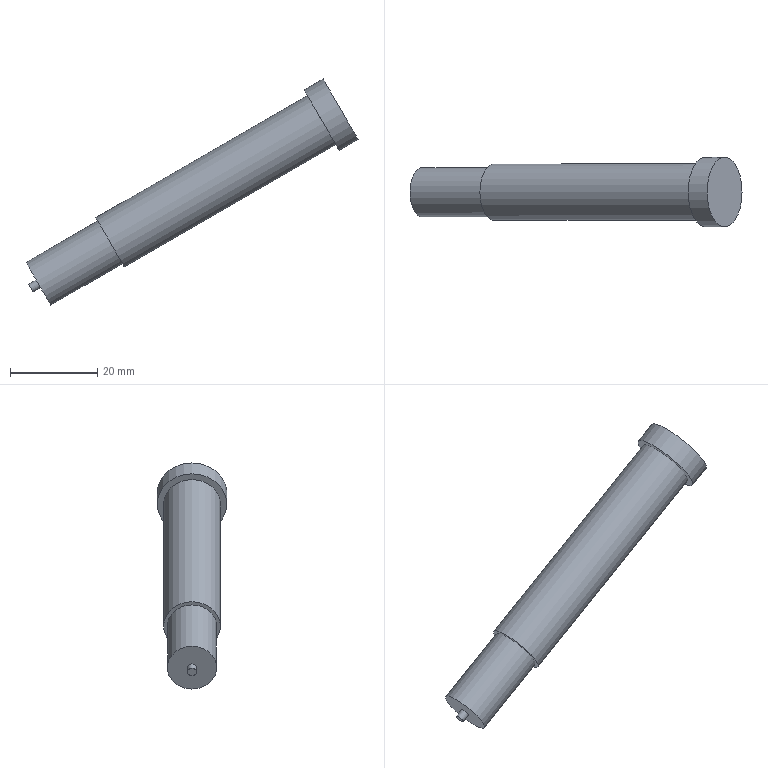Part | NX | features solid 2 | 1 solid | 9 faces | box 76.107 x 16 x 51.821 mm | volume 10350 mm3 | plane 5 | cylinder 4 | commonest cylinder face diameters 2 x1 11.3 x1 13 x1 16 x1
STEP:
#1=CARTESIAN_POINT('',(680.127,-697.825,26.962));
#2=VERTEX_POINT('',#1);
#3=CARTESIAN_POINT('',(683.377,-697.825,21.333));
#4=DIRECTION('',(-0.866,0.00000137,-0.5));
#5=DIRECTION('',(-0.5,0.000000963,0.866));
#6=AXIS2_PLACEMENT_3D('',#3,#4,#5);
#7=CIRCLE('',#6,6.5);
#8=EDGE_CURVE('',#2,#2,#7,.T.);
#9=ORIENTED_EDGE('',*,*,#8,.F.);
#10=EDGE_LOOP('',(#9));
#11=FACE_BOUND('',#10,.T.);
#12=CARTESIAN_POINT('',(728.625,-697.825,54.962));
#13=VERTEX_POINT('',#12);
#14=CARTESIAN_POINT('',(731.875,-697.825,49.333));
#15=DIRECTION('',(-0.866,0.00000137,-0.5));
#16=DIRECTION('',(-0.5,0.000000963,0.866));
#17=AXIS2_PLACEMENT_3D('',#14,#15,#16);
#18=CIRCLE('',#17,6.5);
#19=EDGE_CURVE('',#13,#13,#18,.T.);
#20=ORIENTED_EDGE('',*,*,#19,.T.);
#21=EDGE_LOOP('',(#20));
#22=FACE_BOUND('',#21,.T.);
#23=CARTESIAN_POINT('',(736.205,-697.825,51.833));
#24=DIRECTION('',(-0.866,0.00000137,-0.5));
#25=DIRECTION('',(0.5,-0.000000963,-0.866));
#26=AXIS2_PLACEMENT_3D('',#23,#24,#25);
#27=CYLINDRICAL_SURFACE('',#26,6.5);
#28=ADVANCED_FACE('',(#11,#22),#27,.T.);
#29=CARTESIAN_POINT('',(680.552,-697.825,26.226));
#30=VERTEX_POINT('',#29);
#31=CARTESIAN_POINT('',(683.377,-697.825,21.333));
#32=DIRECTION('',(-0.866,0.00000137,-0.5));
#33=DIRECTION('',(-0.5,0.000000963,0.866));
#34=AXIS2_PLACEMENT_3D('',#31,#32,#33);
#35=CIRCLE('',#34,5.65);
#36=EDGE_CURVE('',#30,#30,#35,.T.);
#37=ORIENTED_EDGE('',*,*,#36,.F.);
#38=EDGE_LOOP('',(#37));
#39=FACE_BOUND('',#38,.T.);
#40=ORIENTED_EDGE('',*,*,#8,.T.);
#41=EDGE_LOOP('',(#40));
#42=FACE_BOUND('',#41,.T.);
#43=CARTESIAN_POINT('',(683.377,-697.825,21.333));
#44=DIRECTION('',(0.866,-0.00000137,0.5));
#45=DIRECTION('',(-0.5,0.000000963,0.866));
#46=AXIS2_PLACEMENT_3D('',#43,#44,#45);
#47=PLANE('',#46);
#48=ADVANCED_FACE('',(#39,#42),#47,.F.);
#49=CARTESIAN_POINT('',(727.875,-697.825,56.261));
#50=VERTEX_POINT('',#49);
#51=CARTESIAN_POINT('',(731.875,-697.825,49.333));
#52=DIRECTION('',(-0.866,0.00000137,-0.5));
#53=DIRECTION('',(-0.5,0.000000963,0.866));
#54=AXIS2_PLACEMENT_3D('',#51,#52,#53);
#55=CIRCLE('',#54,8.);
#56=EDGE_CURVE('',#50,#50,#55,.T.);
#57=ORIENTED_EDGE('',*,*,#56,.T.);
#58=EDGE_LOOP('',(#57));
#59=FACE_BOUND('',#58,.T.);
#60=ORIENTED_EDGE('',*,*,#19,.F.);
#61=EDGE_LOOP('',(#60));
#62=FACE_BOUND('',#61,.T.);
#63=CARTESIAN_POINT('',(731.875,-697.825,49.333));
#64=DIRECTION('',(0.866,-0.00000137,0.5));
#65=DIRECTION('',(-0.5,0.000000963,0.866));
#66=AXIS2_PLACEMENT_3D('',#63,#64,#65);
#67=PLANE('',#66);
#68=ADVANCED_FACE('',(#59,#62),#67,.F.);
#69=ORIENTED_EDGE('',*,*,#56,.F.);
#70=EDGE_LOOP('',(#69));
#71=FACE_BOUND('',#70,.T.);
#72=CARTESIAN_POINT('',(732.205,-697.825,58.761));
#73=VERTEX_POINT('',#72);
#74=CARTESIAN_POINT('',(736.205,-697.825,51.833));
#75=DIRECTION('',(-0.866,0.00000137,-0.5));
#76=DIRECTION('',(-0.5,0.000000963,0.866));
#77=AXIS2_PLACEMENT_3D('',#74,#75,#76);
#78=CIRCLE('',#77,8.);
#79=EDGE_CURVE('',#73,#73,#78,.T.);
#80=ORIENTED_EDGE('',*,*,#79,.T.);
#81=EDGE_LOOP('',(#80));
#82=FACE_BOUND('',#81,.T.);
#83=CARTESIAN_POINT('',(731.875,-697.825,49.333));
#84=DIRECTION('',(0.866,-0.00000137,0.5));
#85=DIRECTION('',(-0.5,0.000000963,0.866));
#86=AXIS2_PLACEMENT_3D('',#83,#84,#85);
#87=CYLINDRICAL_SURFACE('',#86,8.);
#88=ADVANCED_FACE('',(#71,#82),#87,.T.);
#89=ORIENTED_EDGE('',*,*,#79,.F.);
#90=EDGE_LOOP('',(#89));
#91=FACE_BOUND('',#90,.T.);
#92=CARTESIAN_POINT('',(736.205,-697.825,51.833));
#93=DIRECTION('',(0.866,-0.00000137,0.5));
#94=DIRECTION('',(-0.5,0.000000963,0.866));
#95=AXIS2_PLACEMENT_3D('',#92,#93,#94);
#96=PLANE('',#95);
#97=ADVANCED_FACE('',(#91),#96,.T.);
#98=CARTESIAN_POINT('',(664.098,-697.825,16.726));
#99=VERTEX_POINT('',#98);
#100=CARTESIAN_POINT('',(666.923,-697.825,11.833));
#101=DIRECTION('',(-0.866,0.00000137,-0.5));
#102=DIRECTION('',(-0.5,0.000000963,0.866));
#103=AXIS2_PLACEMENT_3D('',#100,#101,#102);
#104=CIRCLE('',#103,5.65);
#105=EDGE_CURVE('',#99,#99,#104,.T.);
#106=ORIENTED_EDGE('',*,*,#105,.F.);
#107=EDGE_LOOP('',(#106));
#108=FACE_BOUND('',#107,.T.);
#109=ORIENTED_EDGE('',*,*,#36,.T.);
#110=EDGE_LOOP('',(#109));
#111=FACE_BOUND('',#110,.T.);
#112=CARTESIAN_POINT('',(666.923,-697.825,11.833));
#113=DIRECTION('',(0.866,-0.00000137,0.5));
#114=DIRECTION('',(-0.5,0.000000963,0.866));
#115=AXIS2_PLACEMENT_3D('',#112,#113,#114);
#116=CYLINDRICAL_SURFACE('',#115,5.65);
#117=ADVANCED_FACE('',(#108,#111),#116,.T.);
#118=CARTESIAN_POINT('',(666.423,-697.825,12.699));
#119=VERTEX_POINT('',#118);
#120=CARTESIAN_POINT('',(666.923,-697.825,11.833));
#121=DIRECTION('',(-0.866,0.00000137,-0.5));
#122=DIRECTION('',(-0.5,0.000000963,0.866));
#123=AXIS2_PLACEMENT_3D('',#120,#121,#122);
#124=CIRCLE('',#123,1.);
#125=EDGE_CURVE('',#119,#119,#124,.T.);
#126=ORIENTED_EDGE('',*,*,#125,.F.);
#127=EDGE_LOOP('',(#126));
#128=FACE_BOUND('',#127,.T.);
#129=ORIENTED_EDGE('',*,*,#105,.T.);
#130=EDGE_LOOP('',(#129));
#131=FACE_BOUND('',#130,.T.);
#132=CARTESIAN_POINT('',(666.923,-697.825,11.833));
#133=DIRECTION('',(0.866,-0.00000137,0.5));
#134=DIRECTION('',(-0.5,0.000000963,0.866));
#135=AXIS2_PLACEMENT_3D('',#132,#133,#134);
#136=PLANE('',#135);
#137=ADVANCED_FACE('',(#128,#131),#136,.F.);
#138=CARTESIAN_POINT('',(664.691,-697.825,11.699));
#139=VERTEX_POINT('',#138);
#140=CARTESIAN_POINT('',(665.191,-697.825,10.833));
#141=DIRECTION('',(-0.866,0.00000137,-0.5));
#142=DIRECTION('',(-0.5,0.000000963,0.866));
#143=AXIS2_PLACEMENT_3D('',#140,#141,#142);
#144=CIRCLE('',#143,1.);
#145=EDGE_CURVE('',#139,#139,#144,.T.);
#146=ORIENTED_EDGE('',*,*,#145,.F.);
#147=EDGE_LOOP('',(#146));
#148=FACE_BOUND('',#147,.T.);
#149=ORIENTED_EDGE('',*,*,#125,.T.);
#150=EDGE_LOOP('',(#149));
#151=FACE_BOUND('',#150,.T.);
#152=CARTESIAN_POINT('',(665.191,-697.825,10.833));
#153=DIRECTION('',(0.866,-0.00000137,0.5));
#154=DIRECTION('',(-0.5,0.000000963,0.866));
#155=AXIS2_PLACEMENT_3D('',#152,#153,#154);
#156=CYLINDRICAL_SURFACE('',#155,1.);
#157=ADVANCED_FACE('',(#148,#151),#156,.T.);
#158=ORIENTED_EDGE('',*,*,#145,.T.);
#159=EDGE_LOOP('',(#158));
#160=FACE_BOUND('',#159,.T.);
#161=CARTESIAN_POINT('',(665.191,-697.825,10.833));
#162=DIRECTION('',(0.866,-0.00000137,0.5));
#163=DIRECTION('',(-0.5,0.000000963,0.866));
#164=AXIS2_PLACEMENT_3D('',#161,#162,#163);
#165=PLANE('',#164);
#166=ADVANCED_FACE('',(#160),#165,.F.);
#167=CLOSED_SHELL('',(#28,#48,#68,#88,#97,#117,#137,#157,#166));
#168=MANIFOLD_SOLID_BREP('',#167);
#169=(LENGTH_UNIT()NAMED_UNIT(*)SI_UNIT(.MILLI.,.METRE.));
#170=UNCERTAINTY_MEASURE_WITH_UNIT(LENGTH_MEASURE(0.00001),#169,'','');
#171=(NAMED_UNIT(*)PLANE_ANGLE_UNIT()SI_UNIT($,.RADIAN.));
#172=(NAMED_UNIT(*)SI_UNIT($,.STERADIAN.)SOLID_ANGLE_UNIT());
#173=(GEOMETRIC_REPRESENTATION_CONTEXT(3)GLOBAL_UNCERTAINTY_ASSIGNED_CONTEXT((#170))GLOBAL_UNIT_ASSIGNED_CONTEXT((#169,#171,#172))REPRESENTATION_CONTEXT('',''));
#174=ADVANCED_BREP_SHAPE_REPRESENTATION('',(#168),#173);